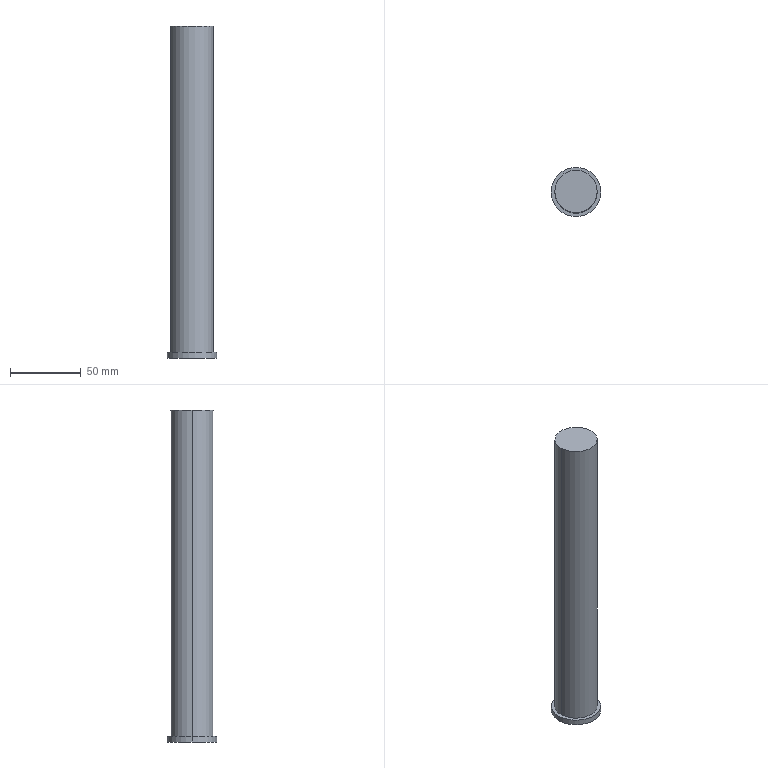Part | SolidWorks | features BaseBody 1 | 1 solid | 11 faces | box 35 x 35 x 235 mm | volume 160759 mm3 | cylinder 6 | plane 3 | cone 2 | commonest cylinder face diameters 14 x2 30 x2 35 x2
STEP:
#1=CARTESIAN_POINT('',(-278.,-175.,-430.5));
#2=VERTEX_POINT('',#1);
#3=CARTESIAN_POINT('',(-264.,-175.,-430.5));
#4=VERTEX_POINT('',#3);
#5=CARTESIAN_POINT('',(-271.,-175.,-430.5));
#6=DIRECTION('',(0.,0.,1.));
#7=DIRECTION('',(1.,0.,0.));
#8=AXIS2_PLACEMENT_3D('',#5,#6,#7);
#9=CIRCLE('',#8,7.);
#10=EDGE_CURVE('',#2,#4,#9,.T.);
#11=ORIENTED_EDGE('',*,*,#10,.F.);
#12=CARTESIAN_POINT('',(-278.,-175.,-390.5));
#13=VERTEX_POINT('',#12);
#14=CARTESIAN_POINT('',(-278.,-175.,-430.5));
#15=DIRECTION('',(0.,0.,1.));
#16=VECTOR('',#15,1000.);
#17=LINE('',#14,#16);
#18=EDGE_CURVE('',#2,#13,#17,.T.);
#19=ORIENTED_EDGE('',*,*,#18,.T.);
#20=CARTESIAN_POINT('',(-264.,-175.,-390.5));
#21=VERTEX_POINT('',#20);
#22=CARTESIAN_POINT('',(-271.,-175.,-390.5));
#23=DIRECTION('',(0.,0.,1.));
#24=DIRECTION('',(1.,0.,0.));
#25=AXIS2_PLACEMENT_3D('',#22,#23,#24);
#26=CIRCLE('',#25,7.);
#27=EDGE_CURVE('',#13,#21,#26,.T.);
#28=ORIENTED_EDGE('',*,*,#27,.T.);
#29=CARTESIAN_POINT('',(-264.,-175.,-430.5));
#30=DIRECTION('',(0.,0.,1.));
#31=VECTOR('',#30,1000.);
#32=LINE('',#29,#31);
#33=EDGE_CURVE('',#4,#21,#32,.T.);
#34=ORIENTED_EDGE('',*,*,#33,.F.);
#35=EDGE_LOOP('',(#11,#19,#28,#34));
#36=FACE_OUTER_BOUND('',#35,.T.);
#37=CARTESIAN_POINT('',(-271.,-175.,-430.5));
#38=DIRECTION('',(0.,0.,1.));
#39=DIRECTION('',(1.,0.,0.));
#40=AXIS2_PLACEMENT_3D('',#37,#38,#39);
#41=CYLINDRICAL_SURFACE('',#40,7.);
#42=ADVANCED_FACE('',(#36),#41,.F.);
#43=CARTESIAN_POINT('',(-271.,-175.,-386.294));
#44=VERTEX_POINT('',#43);
#45=CARTESIAN_POINT('',(-278.,-175.,-390.5));
#46=DIRECTION('',(-0.8572,0.,-0.515));
#47=VECTOR('',#46,1000.);
#48=LINE('',#45,#47);
#49=EDGE_CURVE('',#44,#13,#48,.T.);
#50=ORIENTED_EDGE('',*,*,#49,.F.);
#51=CARTESIAN_POINT('',(-264.,-175.,-390.5));
#52=DIRECTION('',(0.8572,0.,-0.515));
#53=VECTOR('',#52,1000.);
#54=LINE('',#51,#53);
#55=EDGE_CURVE('',#44,#21,#54,.T.);
#56=ORIENTED_EDGE('',*,*,#55,.T.);
#57=ORIENTED_EDGE('',*,*,#27,.F.);
#58=EDGE_LOOP('',(#50,#56,#57));
#59=FACE_OUTER_BOUND('',#58,.T.);
#60=CARTESIAN_POINT('',(-271.,-175.,-390.5));
#61=DIRECTION('',(0.,0.,-1.));
#62=DIRECTION('',(-1.,0.,0.));
#63=AXIS2_PLACEMENT_3D('',#60,#61,#62);
#64=CONICAL_SURFACE('',#63,7.,1.03);
#65=ADVANCED_FACE('',(#59),#64,.F.);
#66=CARTESIAN_POINT('',(-253.5,-175.,-430.5));
#67=VERTEX_POINT('',#66);
#68=CARTESIAN_POINT('',(-288.5,-175.,-430.5));
#69=VERTEX_POINT('',#68);
#70=CARTESIAN_POINT('',(-271.,-175.,-430.5));
#71=DIRECTION('',(0.,0.,-1.));
#72=DIRECTION('',(-1.,0.,0.));
#73=AXIS2_PLACEMENT_3D('',#70,#71,#72);
#74=CIRCLE('',#73,17.5);
#75=EDGE_CURVE('',#67,#69,#74,.T.);
#76=ORIENTED_EDGE('',*,*,#75,.F.);
#77=CARTESIAN_POINT('',(-253.5,-175.,-426.5));
#78=VERTEX_POINT('',#77);
#79=CARTESIAN_POINT('',(-253.5,-175.,-430.5));
#80=DIRECTION('',(0.,0.,1.));
#81=VECTOR('',#80,1000.);
#82=LINE('',#79,#81);
#83=EDGE_CURVE('',#67,#78,#82,.T.);
#84=ORIENTED_EDGE('',*,*,#83,.T.);
#85=CARTESIAN_POINT('',(-288.5,-175.,-426.5));
#86=VERTEX_POINT('',#85);
#87=CARTESIAN_POINT('',(-271.,-175.,-426.5));
#88=DIRECTION('',(0.,0.,-1.));
#89=DIRECTION('',(-1.,0.,0.));
#90=AXIS2_PLACEMENT_3D('',#87,#88,#89);
#91=CIRCLE('',#90,17.5);
#92=EDGE_CURVE('',#78,#86,#91,.T.);
#93=ORIENTED_EDGE('',*,*,#92,.T.);
#94=CARTESIAN_POINT('',(-288.5,-175.,-430.5));
#95=DIRECTION('',(0.,0.,1.));
#96=VECTOR('',#95,1000.);
#97=LINE('',#94,#96);
#98=EDGE_CURVE('',#69,#86,#97,.T.);
#99=ORIENTED_EDGE('',*,*,#98,.F.);
#100=EDGE_LOOP('',(#76,#84,#93,#99));
#101=FACE_OUTER_BOUND('',#100,.T.);
#102=CARTESIAN_POINT('',(-271.,-175.,-430.5));
#103=DIRECTION('',(0.,0.,1.));
#104=DIRECTION('',(-1.,0.,0.));
#105=AXIS2_PLACEMENT_3D('',#102,#103,#104);
#106=CYLINDRICAL_SURFACE('',#105,17.5);
#107=ADVANCED_FACE('',(#101),#106,.T.);
#108=CARTESIAN_POINT('',(-286.,-175.,-426.5));
#109=VERTEX_POINT('',#108);
#110=CARTESIAN_POINT('',(-256.,-175.,-426.5));
#111=VERTEX_POINT('',#110);
#112=CARTESIAN_POINT('',(-271.,-175.,-426.5));
#113=DIRECTION('',(0.,0.,1.));
#114=DIRECTION('',(1.,0.,0.));
#115=AXIS2_PLACEMENT_3D('',#112,#113,#114);
#116=CIRCLE('',#115,15.);
#117=EDGE_CURVE('',#109,#111,#116,.T.);
#118=ORIENTED_EDGE('',*,*,#117,.T.);
#119=CARTESIAN_POINT('',(-256.,-175.,-195.5));
#120=VERTEX_POINT('',#119);
#121=CARTESIAN_POINT('',(-256.,-175.,-430.5));
#122=DIRECTION('',(0.,0.,1.));
#123=VECTOR('',#122,1000.);
#124=LINE('',#121,#123);
#125=EDGE_CURVE('',#111,#120,#124,.T.);
#126=ORIENTED_EDGE('',*,*,#125,.T.);
#127=CARTESIAN_POINT('',(-286.,-175.,-195.5));
#128=VERTEX_POINT('',#127);
#129=CARTESIAN_POINT('',(-271.,-175.,-195.5));
#130=DIRECTION('',(0.,0.,-1.));
#131=DIRECTION('',(-1.,0.,0.));
#132=AXIS2_PLACEMENT_3D('',#129,#130,#131);
#133=CIRCLE('',#132,15.);
#134=EDGE_CURVE('',#120,#128,#133,.T.);
#135=ORIENTED_EDGE('',*,*,#134,.T.);
#136=CARTESIAN_POINT('',(-286.,-175.,-430.5));
#137=DIRECTION('',(0.,0.,1.));
#138=VECTOR('',#137,1000.);
#139=LINE('',#136,#138);
#140=EDGE_CURVE('',#109,#128,#139,.T.);
#141=ORIENTED_EDGE('',*,*,#140,.F.);
#142=EDGE_LOOP('',(#118,#126,#135,#141));
#143=FACE_OUTER_BOUND('',#142,.T.);
#144=CARTESIAN_POINT('',(-271.,-175.,-430.5));
#145=DIRECTION('',(0.,0.,1.));
#146=DIRECTION('',(-1.,0.,0.));
#147=AXIS2_PLACEMENT_3D('',#144,#145,#146);
#148=CYLINDRICAL_SURFACE('',#147,15.);
#149=ADVANCED_FACE('',(#143),#148,.T.);
#150=ORIENTED_EDGE('',*,*,#125,.F.);
#151=CARTESIAN_POINT('',(-271.,-175.,-426.5));
#152=DIRECTION('',(0.,0.,1.));
#153=DIRECTION('',(1.,0.,0.));
#154=AXIS2_PLACEMENT_3D('',#151,#152,#153);
#155=CIRCLE('',#154,15.);
#156=EDGE_CURVE('',#111,#109,#155,.T.);
#157=ORIENTED_EDGE('',*,*,#156,.T.);
#158=ORIENTED_EDGE('',*,*,#140,.T.);
#159=CARTESIAN_POINT('',(-271.,-175.,-195.5));
#160=DIRECTION('',(0.,0.,-1.));
#161=DIRECTION('',(-1.,0.,0.));
#162=AXIS2_PLACEMENT_3D('',#159,#160,#161);
#163=CIRCLE('',#162,15.);
#164=EDGE_CURVE('',#128,#120,#163,.T.);
#165=ORIENTED_EDGE('',*,*,#164,.T.);
#166=EDGE_LOOP('',(#150,#157,#158,#165));
#167=FACE_OUTER_BOUND('',#166,.T.);
#168=CARTESIAN_POINT('',(-271.,-175.,-430.5));
#169=DIRECTION('',(0.,0.,1.));
#170=DIRECTION('',(-1.,0.,0.));
#171=AXIS2_PLACEMENT_3D('',#168,#169,#170);
#172=CYLINDRICAL_SURFACE('',#171,15.);
#173=ADVANCED_FACE('',(#167),#172,.T.);
#174=ORIENTED_EDGE('',*,*,#164,.F.);
#175=ORIENTED_EDGE('',*,*,#134,.F.);
#176=EDGE_LOOP('',(#174,#175));
#177=FACE_OUTER_BOUND('',#176,.T.);
#178=CARTESIAN_POINT('',(-271.,-175.,-195.5));
#179=DIRECTION('',(0.,0.,1.));
#180=DIRECTION('',(-1.,0.,0.));
#181=AXIS2_PLACEMENT_3D('',#178,#179,#180);
#182=PLANE('',#181);
#183=ADVANCED_FACE('',(#177),#182,.T.);
#184=CARTESIAN_POINT('',(-271.,-175.,-426.5));
#185=DIRECTION('',(0.,0.,-1.));
#186=DIRECTION('',(-1.,0.,0.));
#187=AXIS2_PLACEMENT_3D('',#184,#185,#186);
#188=CIRCLE('',#187,17.5);
#189=EDGE_CURVE('',#86,#78,#188,.T.);
#190=ORIENTED_EDGE('',*,*,#189,.F.);
#191=ORIENTED_EDGE('',*,*,#92,.F.);
#192=EDGE_LOOP('',(#190,#191));
#193=FACE_OUTER_BOUND('',#192,.T.);
#194=ORIENTED_EDGE('',*,*,#117,.F.);
#195=ORIENTED_EDGE('',*,*,#156,.F.);
#196=EDGE_LOOP('',(#194,#195));
#197=FACE_BOUND('',#196,.T.);
#198=CARTESIAN_POINT('',(-271.,-175.,-426.5));
#199=DIRECTION('',(0.,0.,-1.));
#200=DIRECTION('',(1.,0.,0.));
#201=AXIS2_PLACEMENT_3D('',#198,#199,#200);
#202=PLANE('',#201);
#203=ADVANCED_FACE('',(#193,#197),#202,.F.);
#204=ORIENTED_EDGE('',*,*,#83,.F.);
#205=CARTESIAN_POINT('',(-271.,-175.,-430.5));
#206=DIRECTION('',(0.,0.,-1.));
#207=DIRECTION('',(-1.,0.,0.));
#208=AXIS2_PLACEMENT_3D('',#205,#206,#207);
#209=CIRCLE('',#208,17.5);
#210=EDGE_CURVE('',#69,#67,#209,.T.);
#211=ORIENTED_EDGE('',*,*,#210,.F.);
#212=ORIENTED_EDGE('',*,*,#98,.T.);
#213=ORIENTED_EDGE('',*,*,#189,.T.);
#214=EDGE_LOOP('',(#204,#211,#212,#213));
#215=FACE_OUTER_BOUND('',#214,.T.);
#216=CARTESIAN_POINT('',(-271.,-175.,-430.5));
#217=DIRECTION('',(0.,0.,1.));
#218=DIRECTION('',(-1.,0.,0.));
#219=AXIS2_PLACEMENT_3D('',#216,#217,#218);
#220=CYLINDRICAL_SURFACE('',#219,17.5);
#221=ADVANCED_FACE('',(#215),#220,.T.);
#222=CARTESIAN_POINT('',(-271.,-175.,-430.5));
#223=DIRECTION('',(0.,0.,1.));
#224=DIRECTION('',(1.,0.,0.));
#225=AXIS2_PLACEMENT_3D('',#222,#223,#224);
#226=CIRCLE('',#225,7.);
#227=EDGE_CURVE('',#4,#2,#226,.T.);
#228=ORIENTED_EDGE('',*,*,#227,.T.);
#229=ORIENTED_EDGE('',*,*,#10,.T.);
#230=EDGE_LOOP('',(#228,#229));
#231=FACE_BOUND('',#230,.T.);
#232=ORIENTED_EDGE('',*,*,#210,.T.);
#233=ORIENTED_EDGE('',*,*,#75,.T.);
#234=EDGE_LOOP('',(#232,#233));
#235=FACE_OUTER_BOUND('',#234,.T.);
#236=CARTESIAN_POINT('',(-271.,-175.,-430.5));
#237=DIRECTION('',(0.,0.,1.));
#238=DIRECTION('',(-1.,0.,0.));
#239=AXIS2_PLACEMENT_3D('',#236,#237,#238);
#240=PLANE('',#239);
#241=ADVANCED_FACE('',(#231,#235),#240,.F.);
#242=ORIENTED_EDGE('',*,*,#55,.F.);
#243=ORIENTED_EDGE('',*,*,#49,.T.);
#244=CARTESIAN_POINT('',(-271.,-175.,-390.5));
#245=DIRECTION('',(0.,0.,1.));
#246=DIRECTION('',(1.,0.,0.));
#247=AXIS2_PLACEMENT_3D('',#244,#245,#246);
#248=CIRCLE('',#247,7.);
#249=EDGE_CURVE('',#21,#13,#248,.T.);
#250=ORIENTED_EDGE('',*,*,#249,.F.);
#251=EDGE_LOOP('',(#242,#243,#250));
#252=FACE_OUTER_BOUND('',#251,.T.);
#253=CARTESIAN_POINT('',(-271.,-175.,-390.5));
#254=DIRECTION('',(0.,0.,-1.));
#255=DIRECTION('',(-1.,0.,0.));
#256=AXIS2_PLACEMENT_3D('',#253,#254,#255);
#257=CONICAL_SURFACE('',#256,7.,1.03);
#258=ADVANCED_FACE('',(#252),#257,.F.);
#259=ORIENTED_EDGE('',*,*,#18,.F.);
#260=ORIENTED_EDGE('',*,*,#227,.F.);
#261=ORIENTED_EDGE('',*,*,#33,.T.);
#262=ORIENTED_EDGE('',*,*,#249,.T.);
#263=EDGE_LOOP('',(#259,#260,#261,#262));
#264=FACE_OUTER_BOUND('',#263,.T.);
#265=CARTESIAN_POINT('',(-271.,-175.,-430.5));
#266=DIRECTION('',(0.,0.,1.));
#267=DIRECTION('',(1.,0.,0.));
#268=AXIS2_PLACEMENT_3D('',#265,#266,#267);
#269=CYLINDRICAL_SURFACE('',#268,7.);
#270=ADVANCED_FACE('',(#264),#269,.F.);
#271=CLOSED_SHELL('',(#42,#65,#107,#149,#173,#183,#203,#221,#241,#258,#270));
#272=MANIFOLD_SOLID_BREP('',#271);
#273=CARTESIAN_POINT('',(0.,0.,0.));
#274=DIRECTION('',(0.,0.,1.));
#275=DIRECTION('',(1.,0.,0.));
#276=AXIS2_PLACEMENT_3D('',#273,#274,#275);
#277=(LENGTH_UNIT()NAMED_UNIT(*)SI_UNIT(.MILLI.,.METRE.));
#278=UNCERTAINTY_MEASURE_WITH_UNIT(LENGTH_MEASURE(0.00001),#277,'','');
#279=(NAMED_UNIT(*)PLANE_ANGLE_UNIT()SI_UNIT($,.RADIAN.));
#280=(NAMED_UNIT(*)SI_UNIT($,.STERADIAN.)SOLID_ANGLE_UNIT());
#281=(GEOMETRIC_REPRESENTATION_CONTEXT(3)GLOBAL_UNCERTAINTY_ASSIGNED_CONTEXT((#278))GLOBAL_UNIT_ASSIGNED_CONTEXT((#277,#279,#280))REPRESENTATION_CONTEXT('',''));
#282=ADVANCED_BREP_SHAPE_REPRESENTATION('',(#272,#276),#281);